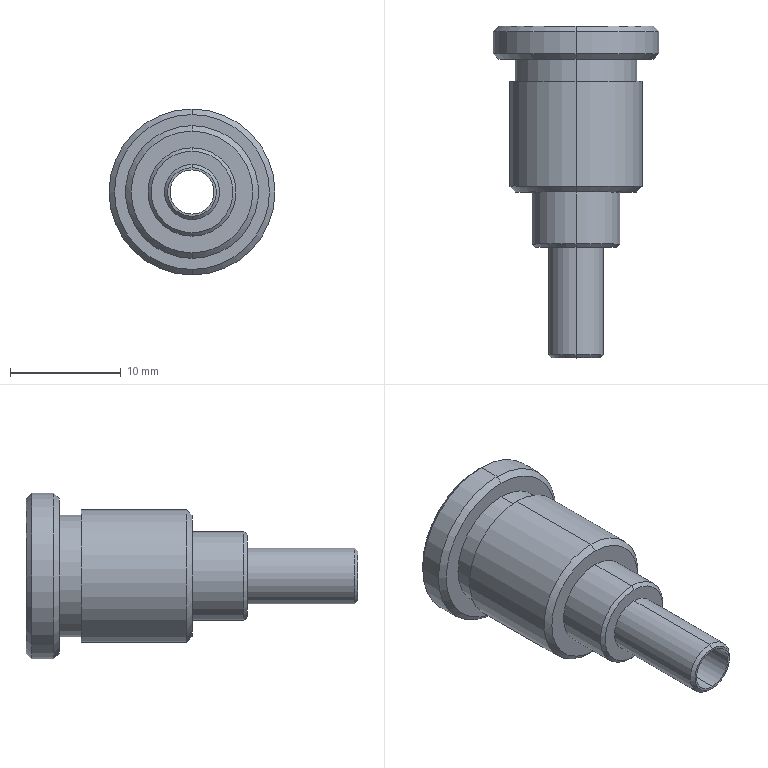Part | SolidWorks | features Chamfer 6, ICE 5, Extrusion 1, RevCut 1 | 1 solid | 30 faces | box 15 x 30 x 15 mm | volume 1897 mm3 | cylinder 12 | cone 12 | plane 6 | commonest cylinder face diameters 4 x2 5 x2 8 x2 11 x2 12 x2 15 x2
STEP:
#1=CARTESIAN_POINT('',(0.,-3.,-5.5));
#2=VERTEX_POINT('',#1);
#3=CARTESIAN_POINT('',(0.,-3.,5.5));
#4=VERTEX_POINT('',#3);
#5=CARTESIAN_POINT('',(0.,-3.,0.));
#6=DIRECTION('',(0.,-1.,0.));
#7=DIRECTION('',(0.,0.,-1.));
#8=AXIS2_PLACEMENT_3D('',#5,#6,#7);
#9=CIRCLE('',#8,5.5);
#10=EDGE_CURVE('',#2,#4,#9,.T.);
#11=ORIENTED_EDGE('',*,*,#10,.T.);
#12=CARTESIAN_POINT('',(0.,-5.,5.5));
#13=VERTEX_POINT('',#12);
#14=CARTESIAN_POINT('',(0.,-14.5,5.5));
#15=DIRECTION('',(0.,-1.,0.));
#16=VECTOR('',#15,1000.);
#17=LINE('',#14,#16);
#18=EDGE_CURVE('',#4,#13,#17,.T.);
#19=ORIENTED_EDGE('',*,*,#18,.T.);
#20=CARTESIAN_POINT('',(0.,-5.,-5.5));
#21=VERTEX_POINT('',#20);
#22=CARTESIAN_POINT('',(0.,-5.,0.));
#23=DIRECTION('',(0.,-1.,0.));
#24=DIRECTION('',(0.,0.,-1.));
#25=AXIS2_PLACEMENT_3D('',#22,#23,#24);
#26=CIRCLE('',#25,5.5);
#27=EDGE_CURVE('',#21,#13,#26,.T.);
#28=ORIENTED_EDGE('',*,*,#27,.F.);
#29=CARTESIAN_POINT('',(0.,-14.5,-5.5));
#30=DIRECTION('',(0.,-1.,0.));
#31=VECTOR('',#30,1000.);
#32=LINE('',#29,#31);
#33=EDGE_CURVE('',#2,#21,#32,.T.);
#34=ORIENTED_EDGE('',*,*,#33,.F.);
#35=EDGE_LOOP('',(#11,#19,#28,#34));
#36=FACE_OUTER_BOUND('',#35,.T.);
#37=CARTESIAN_POINT('',(0.,-14.5,0.));
#38=DIRECTION('',(0.,-1.,0.));
#39=DIRECTION('',(0.,0.,-1.));
#40=AXIS2_PLACEMENT_3D('',#37,#38,#39);
#41=CYLINDRICAL_SURFACE('',#40,5.5);
#42=ADVANCED_FACE('',(#36),#41,.T.);
#43=CARTESIAN_POINT('',(0.,-30.,-2.2));
#44=VERTEX_POINT('',#43);
#45=CARTESIAN_POINT('',(0.,-30.,2.2));
#46=VERTEX_POINT('',#45);
#47=CARTESIAN_POINT('',(0.,-30.,0.));
#48=DIRECTION('',(0.,-1.,0.));
#49=DIRECTION('',(0.,0.,-1.));
#50=AXIS2_PLACEMENT_3D('',#47,#48,#49);
#51=CIRCLE('',#50,2.2);
#52=EDGE_CURVE('',#44,#46,#51,.T.);
#53=ORIENTED_EDGE('',*,*,#52,.F.);
#54=CARTESIAN_POINT('',(0.,-29.7,-2.5));
#55=VERTEX_POINT('',#54);
#56=CARTESIAN_POINT('',(0.,-30.,-2.2));
#57=DIRECTION('',(0.,0.7071,-0.7071));
#58=VECTOR('',#57,1000.);
#59=LINE('',#56,#58);
#60=EDGE_CURVE('',#44,#55,#59,.T.);
#61=ORIENTED_EDGE('',*,*,#60,.T.);
#62=CARTESIAN_POINT('',(0.,-29.7,2.5));
#63=VERTEX_POINT('',#62);
#64=CARTESIAN_POINT('',(0.,-29.7,0.));
#65=DIRECTION('',(0.,1.,0.));
#66=DIRECTION('',(0.,0.,-1.));
#67=AXIS2_PLACEMENT_3D('',#64,#65,#66);
#68=CIRCLE('',#67,2.5);
#69=EDGE_CURVE('',#63,#55,#68,.T.);
#70=ORIENTED_EDGE('',*,*,#69,.F.);
#71=CARTESIAN_POINT('',(0.,-30.,2.2));
#72=DIRECTION('',(0.,0.7071,0.7071));
#73=VECTOR('',#72,1000.);
#74=LINE('',#71,#73);
#75=EDGE_CURVE('',#46,#63,#74,.T.);
#76=ORIENTED_EDGE('',*,*,#75,.F.);
#77=EDGE_LOOP('',(#53,#61,#70,#76));
#78=FACE_OUTER_BOUND('',#77,.T.);
#79=CARTESIAN_POINT('',(0.,-30.,0.));
#80=DIRECTION('',(0.,1.,0.));
#81=DIRECTION('',(0.,0.,1.));
#82=AXIS2_PLACEMENT_3D('',#79,#80,#81);
#83=CONICAL_SURFACE('',#82,2.2,0.7854);
#84=ADVANCED_FACE('',(#78),#83,.T.);
#85=CARTESIAN_POINT('',(0.,-20.,-3.7));
#86=VERTEX_POINT('',#85);
#87=CARTESIAN_POINT('',(0.,-20.,3.7));
#88=VERTEX_POINT('',#87);
#89=CARTESIAN_POINT('',(0.,-20.,0.));
#90=DIRECTION('',(0.,-1.,0.));
#91=DIRECTION('',(0.,0.,-1.));
#92=AXIS2_PLACEMENT_3D('',#89,#90,#91);
#93=CIRCLE('',#92,3.7);
#94=EDGE_CURVE('',#86,#88,#93,.T.);
#95=ORIENTED_EDGE('',*,*,#94,.F.);
#96=CARTESIAN_POINT('',(0.,-19.7,-4.));
#97=VERTEX_POINT('',#96);
#98=CARTESIAN_POINT('',(0.,-20.,-3.7));
#99=DIRECTION('',(0.,0.7071,-0.7071));
#100=VECTOR('',#99,1000.);
#101=LINE('',#98,#100);
#102=EDGE_CURVE('',#86,#97,#101,.T.);
#103=ORIENTED_EDGE('',*,*,#102,.T.);
#104=CARTESIAN_POINT('',(0.,-19.7,4.));
#105=VERTEX_POINT('',#104);
#106=CARTESIAN_POINT('',(0.,-19.7,0.));
#107=DIRECTION('',(0.,1.,0.));
#108=DIRECTION('',(0.,0.,-1.));
#109=AXIS2_PLACEMENT_3D('',#106,#107,#108);
#110=CIRCLE('',#109,4.);
#111=EDGE_CURVE('',#105,#97,#110,.T.);
#112=ORIENTED_EDGE('',*,*,#111,.F.);
#113=CARTESIAN_POINT('',(0.,-20.,3.7));
#114=DIRECTION('',(0.,0.7071,0.7071));
#115=VECTOR('',#114,1000.);
#116=LINE('',#113,#115);
#117=EDGE_CURVE('',#88,#105,#116,.T.);
#118=ORIENTED_EDGE('',*,*,#117,.F.);
#119=EDGE_LOOP('',(#95,#103,#112,#118));
#120=FACE_OUTER_BOUND('',#119,.T.);
#121=CARTESIAN_POINT('',(0.,-20.,0.));
#122=DIRECTION('',(0.,1.,0.));
#123=DIRECTION('',(0.,0.,1.));
#124=AXIS2_PLACEMENT_3D('',#121,#122,#123);
#125=CONICAL_SURFACE('',#124,3.7,0.7854);
#126=ADVANCED_FACE('',(#120),#125,.T.);
#127=ORIENTED_EDGE('',*,*,#111,.T.);
#128=CARTESIAN_POINT('',(0.,-15.,-4.));
#129=VERTEX_POINT('',#128);
#130=CARTESIAN_POINT('',(0.,-20.,-4.));
#131=DIRECTION('',(0.,1.,0.));
#132=VECTOR('',#131,1000.);
#133=LINE('',#130,#132);
#134=EDGE_CURVE('',#97,#129,#133,.T.);
#135=ORIENTED_EDGE('',*,*,#134,.T.);
#136=CARTESIAN_POINT('',(0.,-15.,4.));
#137=VERTEX_POINT('',#136);
#138=CARTESIAN_POINT('',(0.,-15.,0.));
#139=DIRECTION('',(0.,-1.,0.));
#140=DIRECTION('',(0.,0.,1.));
#141=AXIS2_PLACEMENT_3D('',#138,#139,#140);
#142=CIRCLE('',#141,4.);
#143=EDGE_CURVE('',#129,#137,#142,.T.);
#144=ORIENTED_EDGE('',*,*,#143,.T.);
#145=CARTESIAN_POINT('',(0.,-20.,4.));
#146=DIRECTION('',(0.,1.,0.));
#147=VECTOR('',#146,1000.);
#148=LINE('',#145,#147);
#149=EDGE_CURVE('',#105,#137,#148,.T.);
#150=ORIENTED_EDGE('',*,*,#149,.F.);
#151=EDGE_LOOP('',(#127,#135,#144,#150));
#152=FACE_OUTER_BOUND('',#151,.T.);
#153=CARTESIAN_POINT('',(0.,-20.,0.));
#154=DIRECTION('',(0.,1.,0.));
#155=DIRECTION('',(0.,0.,1.));
#156=AXIS2_PLACEMENT_3D('',#153,#154,#155);
#157=CYLINDRICAL_SURFACE('',#156,4.);
#158=ADVANCED_FACE('',(#152),#157,.T.);
#159=CARTESIAN_POINT('',(0.,-3.,-7.));
#160=VERTEX_POINT('',#159);
#161=CARTESIAN_POINT('',(0.,-3.,7.));
#162=VERTEX_POINT('',#161);
#163=CARTESIAN_POINT('',(0.,-3.,0.));
#164=DIRECTION('',(0.,-1.,0.));
#165=DIRECTION('',(0.,0.,1.));
#166=AXIS2_PLACEMENT_3D('',#163,#164,#165);
#167=CIRCLE('',#166,7.);
#168=EDGE_CURVE('',#160,#162,#167,.T.);
#169=ORIENTED_EDGE('',*,*,#168,.F.);
#170=CARTESIAN_POINT('',(0.,-2.5,-7.5));
#171=VERTEX_POINT('',#170);
#172=CARTESIAN_POINT('',(0.,-2.5,-7.5));
#173=DIRECTION('',(0.,0.7071,-0.7071));
#174=VECTOR('',#173,1000.);
#175=LINE('',#172,#174);
#176=EDGE_CURVE('',#160,#171,#175,.T.);
#177=ORIENTED_EDGE('',*,*,#176,.T.);
#178=CARTESIAN_POINT('',(0.,-2.5,7.5));
#179=VERTEX_POINT('',#178);
#180=CARTESIAN_POINT('',(0.,-2.5,0.));
#181=DIRECTION('',(0.,1.,0.));
#182=DIRECTION('',(0.,0.,1.));
#183=AXIS2_PLACEMENT_3D('',#180,#181,#182);
#184=CIRCLE('',#183,7.5);
#185=EDGE_CURVE('',#179,#171,#184,.T.);
#186=ORIENTED_EDGE('',*,*,#185,.F.);
#187=CARTESIAN_POINT('',(0.,-2.5,7.5));
#188=DIRECTION('',(0.,0.7071,0.7071));
#189=VECTOR('',#188,1000.);
#190=LINE('',#187,#189);
#191=EDGE_CURVE('',#162,#179,#190,.T.);
#192=ORIENTED_EDGE('',*,*,#191,.F.);
#193=EDGE_LOOP('',(#169,#177,#186,#192));
#194=FACE_OUTER_BOUND('',#193,.T.);
#195=CARTESIAN_POINT('',(0.,-2.5,0.));
#196=DIRECTION('',(0.,1.,0.));
#197=DIRECTION('',(0.,0.,1.));
#198=AXIS2_PLACEMENT_3D('',#195,#196,#197);
#199=CONICAL_SURFACE('',#198,7.5,0.7854);
#200=ADVANCED_FACE('',(#194),#199,.T.);
#201=CARTESIAN_POINT('',(0.,0.,7.));
#202=VERTEX_POINT('',#201);
#203=CARTESIAN_POINT('',(0.,0.,-7.));
#204=VERTEX_POINT('',#203);
#205=CARTESIAN_POINT('',(0.,0.,0.));
#206=DIRECTION('',(0.,1.,0.));
#207=DIRECTION('',(0.,0.,1.));
#208=AXIS2_PLACEMENT_3D('',#205,#206,#207);
#209=CIRCLE('',#208,7.);
#210=EDGE_CURVE('',#202,#204,#209,.T.);
#211=ORIENTED_EDGE('',*,*,#210,.F.);
#212=CARTESIAN_POINT('',(0.,-0.5,7.5));
#213=VERTEX_POINT('',#212);
#214=CARTESIAN_POINT('',(0.,0.,7.));
#215=DIRECTION('',(0.,-0.7071,0.7071));
#216=VECTOR('',#215,1000.);
#217=LINE('',#214,#216);
#218=EDGE_CURVE('',#202,#213,#217,.T.);
#219=ORIENTED_EDGE('',*,*,#218,.T.);
#220=CARTESIAN_POINT('',(0.,-0.5,-7.5));
#221=VERTEX_POINT('',#220);
#222=CARTESIAN_POINT('',(0.,-0.5,0.));
#223=DIRECTION('',(0.,-1.,0.));
#224=DIRECTION('',(0.,0.,1.));
#225=AXIS2_PLACEMENT_3D('',#222,#223,#224);
#226=CIRCLE('',#225,7.5);
#227=EDGE_CURVE('',#221,#213,#226,.T.);
#228=ORIENTED_EDGE('',*,*,#227,.F.);
#229=CARTESIAN_POINT('',(0.,0.,-7.));
#230=DIRECTION('',(0.,-0.7071,-0.7071));
#231=VECTOR('',#230,1000.);
#232=LINE('',#229,#231);
#233=EDGE_CURVE('',#204,#221,#232,.T.);
#234=ORIENTED_EDGE('',*,*,#233,.F.);
#235=EDGE_LOOP('',(#211,#219,#228,#234));
#236=FACE_OUTER_BOUND('',#235,.T.);
#237=CARTESIAN_POINT('',(0.,0.,0.));
#238=DIRECTION('',(0.,-1.,0.));
#239=DIRECTION('',(0.,0.,-1.));
#240=AXIS2_PLACEMENT_3D('',#237,#238,#239);
#241=CONICAL_SURFACE('',#240,7.,0.7854);
#242=ADVANCED_FACE('',(#236),#241,.T.);
#243=CARTESIAN_POINT('',(0.,-1.,-2.));
#244=VERTEX_POINT('',#243);
#245=CARTESIAN_POINT('',(0.,-1.,2.));
#246=VERTEX_POINT('',#245);
#247=CARTESIAN_POINT('',(0.,-1.,0.));
#248=DIRECTION('',(0.,1.,0.));
#249=DIRECTION('',(0.,0.,1.));
#250=AXIS2_PLACEMENT_3D('',#247,#248,#249);
#251=CIRCLE('',#250,2.);
#252=EDGE_CURVE('',#244,#246,#251,.T.);
#253=ORIENTED_EDGE('',*,*,#252,.F.);
#254=CARTESIAN_POINT('',(0.,0.,-3.));
#255=VERTEX_POINT('',#254);
#256=CARTESIAN_POINT('',(0.,-1.,-2.));
#257=DIRECTION('',(0.,0.7071,-0.7071));
#258=VECTOR('',#257,1000.);
#259=LINE('',#256,#258);
#260=EDGE_CURVE('',#244,#255,#259,.T.);
#261=ORIENTED_EDGE('',*,*,#260,.T.);
#262=CARTESIAN_POINT('',(0.,0.,3.));
#263=VERTEX_POINT('',#262);
#264=CARTESIAN_POINT('',(0.,0.,0.));
#265=DIRECTION('',(0.,-1.,0.));
#266=DIRECTION('',(0.,0.,1.));
#267=AXIS2_PLACEMENT_3D('',#264,#265,#266);
#268=CIRCLE('',#267,3.);
#269=EDGE_CURVE('',#263,#255,#268,.T.);
#270=ORIENTED_EDGE('',*,*,#269,.F.);
#271=CARTESIAN_POINT('',(0.,-1.,2.));
#272=DIRECTION('',(0.,0.7071,0.7071));
#273=VECTOR('',#272,1000.);
#274=LINE('',#271,#273);
#275=EDGE_CURVE('',#246,#263,#274,.T.);
#276=ORIENTED_EDGE('',*,*,#275,.F.);
#277=EDGE_LOOP('',(#253,#261,#270,#276));
#278=FACE_OUTER_BOUND('',#277,.T.);
#279=CARTESIAN_POINT('',(0.,-1.,0.));
#280=DIRECTION('',(0.,1.,0.));
#281=DIRECTION('',(0.,0.,1.));
#282=AXIS2_PLACEMENT_3D('',#279,#280,#281);
#283=CONICAL_SURFACE('',#282,2.,0.7854);
#284=ADVANCED_FACE('',(#278),#283,.F.);
#285=ORIENTED_EDGE('',*,*,#185,.T.);
#286=CARTESIAN_POINT('',(0.,-3.,-7.5));
#287=DIRECTION('',(0.,1.,0.));
#288=VECTOR('',#287,1000.);
#289=LINE('',#286,#288);
#290=EDGE_CURVE('',#171,#221,#289,.T.);
#291=ORIENTED_EDGE('',*,*,#290,.T.);
#292=ORIENTED_EDGE('',*,*,#227,.T.);
#293=CARTESIAN_POINT('',(0.,-3.,7.5));
#294=DIRECTION('',(0.,1.,0.));
#295=VECTOR('',#294,1000.);
#296=LINE('',#293,#295);
#297=EDGE_CURVE('',#179,#213,#296,.T.);
#298=ORIENTED_EDGE('',*,*,#297,.F.);
#299=EDGE_LOOP('',(#285,#291,#292,#298));
#300=FACE_OUTER_BOUND('',#299,.T.);
#301=CARTESIAN_POINT('',(0.,-3.,0.));
#302=DIRECTION('',(0.,1.,0.));
#303=DIRECTION('',(0.,0.,1.));
#304=AXIS2_PLACEMENT_3D('',#301,#302,#303);
#305=CYLINDRICAL_SURFACE('',#304,7.5);
#306=ADVANCED_FACE('',(#300),#305,.T.);
#307=CARTESIAN_POINT('',(0.,-15.,-5.5));
#308=VERTEX_POINT('',#307);
#309=CARTESIAN_POINT('',(0.,-15.,5.5));
#310=VERTEX_POINT('',#309);
#311=CARTESIAN_POINT('',(0.,-15.,0.));
#312=DIRECTION('',(0.,-1.,0.));
#313=DIRECTION('',(0.,0.,1.));
#314=AXIS2_PLACEMENT_3D('',#311,#312,#313);
#315=CIRCLE('',#314,5.5);
#316=EDGE_CURVE('',#308,#310,#315,.T.);
#317=ORIENTED_EDGE('',*,*,#316,.F.);
#318=CARTESIAN_POINT('',(0.,-14.5,-6.));
#319=VERTEX_POINT('',#318);
#320=CARTESIAN_POINT('',(0.,-14.5,-6.));
#321=DIRECTION('',(0.,0.7071,-0.7071));
#322=VECTOR('',#321,1000.);
#323=LINE('',#320,#322);
#324=EDGE_CURVE('',#308,#319,#323,.T.);
#325=ORIENTED_EDGE('',*,*,#324,.T.);
#326=CARTESIAN_POINT('',(0.,-14.5,6.));
#327=VERTEX_POINT('',#326);
#328=CARTESIAN_POINT('',(0.,-14.5,0.));
#329=DIRECTION('',(0.,1.,0.));
#330=DIRECTION('',(0.,0.,1.));
#331=AXIS2_PLACEMENT_3D('',#328,#329,#330);
#332=CIRCLE('',#331,6.);
#333=EDGE_CURVE('',#327,#319,#332,.T.);
#334=ORIENTED_EDGE('',*,*,#333,.F.);
#335=CARTESIAN_POINT('',(0.,-14.5,6.));
#336=DIRECTION('',(0.,0.7071,0.7071));
#337=VECTOR('',#336,1000.);
#338=LINE('',#335,#337);
#339=EDGE_CURVE('',#310,#327,#338,.T.);
#340=ORIENTED_EDGE('',*,*,#339,.F.);
#341=EDGE_LOOP('',(#317,#325,#334,#340));
#342=FACE_OUTER_BOUND('',#341,.T.);
#343=CARTESIAN_POINT('',(0.,-14.5,0.));
#344=DIRECTION('',(0.,1.,0.));
#345=DIRECTION('',(0.,0.,1.));
#346=AXIS2_PLACEMENT_3D('',#343,#344,#345);
#347=CONICAL_SURFACE('',#346,6.,0.7854);
#348=ADVANCED_FACE('',(#342),#347,.T.);
#349=CARTESIAN_POINT('',(0.,-30.,-2.));
#350=VERTEX_POINT('',#349);
#351=CARTESIAN_POINT('',(0.,-30.,2.));
#352=VERTEX_POINT('',#351);
#353=CARTESIAN_POINT('',(0.,-30.,0.));
#354=DIRECTION('',(0.,1.,0.));
#355=DIRECTION('',(0.,0.,1.));
#356=AXIS2_PLACEMENT_3D('',#353,#354,#355);
#357=CIRCLE('',#356,2.);
#358=EDGE_CURVE('',#350,#352,#357,.T.);
#359=ORIENTED_EDGE('',*,*,#358,.F.);
#360=CARTESIAN_POINT('',(0.,-30.,-2.));
#361=DIRECTION('',(0.,1.,0.));
#362=VECTOR('',#361,1000.);
#363=LINE('',#360,#362);
#364=EDGE_CURVE('',#350,#244,#363,.T.);
#365=ORIENTED_EDGE('',*,*,#364,.T.);
#366=ORIENTED_EDGE('',*,*,#252,.T.);
#367=CARTESIAN_POINT('',(0.,-30.,2.));
#368=DIRECTION('',(0.,1.,0.));
#369=VECTOR('',#368,1000.);
#370=LINE('',#367,#369);
#371=EDGE_CURVE('',#352,#246,#370,.T.);
#372=ORIENTED_EDGE('',*,*,#371,.F.);
#373=EDGE_LOOP('',(#359,#365,#366,#372));
#374=FACE_OUTER_BOUND('',#373,.T.);
#375=CARTESIAN_POINT('',(0.,-30.,0.));
#376=DIRECTION('',(0.,1.,0.));
#377=DIRECTION('',(0.,0.,1.));
#378=AXIS2_PLACEMENT_3D('',#375,#376,#377);
#379=CYLINDRICAL_SURFACE('',#378,2.);
#380=ADVANCED_FACE('',(#374),#379,.F.);
#381=ORIENTED_EDGE('',*,*,#69,.T.);
#382=CARTESIAN_POINT('',(0.,-20.,-2.5));
#383=VERTEX_POINT('',#382);
#384=CARTESIAN_POINT('',(0.,-30.,-2.5));
#385=DIRECTION('',(0.,1.,0.));
#386=VECTOR('',#385,1000.);
#387=LINE('',#384,#386);
#388=EDGE_CURVE('',#55,#383,#387,.T.);
#389=ORIENTED_EDGE('',*,*,#388,.T.);
#390=CARTESIAN_POINT('',(0.,-20.,2.5));
#391=VERTEX_POINT('',#390);
#392=CARTESIAN_POINT('',(0.,-20.,0.));
#393=DIRECTION('',(0.,-1.,0.));
#394=DIRECTION('',(0.,0.,-1.));
#395=AXIS2_PLACEMENT_3D('',#392,#393,#394);
#396=CIRCLE('',#395,2.5);
#397=EDGE_CURVE('',#383,#391,#396,.T.);
#398=ORIENTED_EDGE('',*,*,#397,.T.);
#399=CARTESIAN_POINT('',(0.,-30.,2.5));
#400=DIRECTION('',(0.,1.,0.));
#401=VECTOR('',#400,1000.);
#402=LINE('',#399,#401);
#403=EDGE_CURVE('',#63,#391,#402,.T.);
#404=ORIENTED_EDGE('',*,*,#403,.F.);
#405=EDGE_LOOP('',(#381,#389,#398,#404));
#406=FACE_OUTER_BOUND('',#405,.T.);
#407=CARTESIAN_POINT('',(0.,-30.,0.));
#408=DIRECTION('',(0.,1.,0.));
#409=DIRECTION('',(0.,0.,1.));
#410=AXIS2_PLACEMENT_3D('',#407,#408,#409);
#411=CYLINDRICAL_SURFACE('',#410,2.5);
#412=ADVANCED_FACE('',(#406),#411,.T.);
#413=ORIENTED_EDGE('',*,*,#333,.T.);
#414=CARTESIAN_POINT('',(0.,-5.,-6.));
#415=VERTEX_POINT('',#414);
#416=CARTESIAN_POINT('',(0.,-15.,-6.));
#417=DIRECTION('',(0.,1.,0.));
#418=VECTOR('',#417,1000.);
#419=LINE('',#416,#418);
#420=EDGE_CURVE('',#319,#415,#419,.T.);
#421=ORIENTED_EDGE('',*,*,#420,.T.);
#422=CARTESIAN_POINT('',(0.,-5.,6.));
#423=VERTEX_POINT('',#422);
#424=CARTESIAN_POINT('',(0.,-5.,0.));
#425=DIRECTION('',(0.,-1.,0.));
#426=DIRECTION('',(0.,0.,1.));
#427=AXIS2_PLACEMENT_3D('',#424,#425,#426);
#428=CIRCLE('',#427,6.);
#429=EDGE_CURVE('',#415,#423,#428,.T.);
#430=ORIENTED_EDGE('',*,*,#429,.T.);
#431=CARTESIAN_POINT('',(0.,-15.,6.));
#432=DIRECTION('',(0.,1.,0.));
#433=VECTOR('',#432,1000.);
#434=LINE('',#431,#433);
#435=EDGE_CURVE('',#327,#423,#434,.T.);
#436=ORIENTED_EDGE('',*,*,#435,.F.);
#437=EDGE_LOOP('',(#413,#421,#430,#436));
#438=FACE_OUTER_BOUND('',#437,.T.);
#439=CARTESIAN_POINT('',(0.,-15.,0.));
#440=DIRECTION('',(0.,1.,0.));
#441=DIRECTION('',(0.,0.,1.));
#442=AXIS2_PLACEMENT_3D('',#439,#440,#441);
#443=CYLINDRICAL_SURFACE('',#442,6.);
#444=ADVANCED_FACE('',(#438),#443,.T.);
#445=ORIENTED_EDGE('',*,*,#420,.F.);
#446=CARTESIAN_POINT('',(0.,-14.5,0.));
#447=DIRECTION('',(0.,1.,0.));
#448=DIRECTION('',(0.,0.,1.));
#449=AXIS2_PLACEMENT_3D('',#446,#447,#448);
#450=CIRCLE('',#449,6.);
#451=EDGE_CURVE('',#319,#327,#450,.T.);
#452=ORIENTED_EDGE('',*,*,#451,.T.);
#453=ORIENTED_EDGE('',*,*,#435,.T.);
#454=CARTESIAN_POINT('',(0.,-5.,0.));
#455=DIRECTION('',(0.,-1.,0.));
#456=DIRECTION('',(0.,0.,1.));
#457=AXIS2_PLACEMENT_3D('',#454,#455,#456);
#458=CIRCLE('',#457,6.);
#459=EDGE_CURVE('',#423,#415,#458,.T.);
#460=ORIENTED_EDGE('',*,*,#459,.T.);
#461=EDGE_LOOP('',(#445,#452,#453,#460));
#462=FACE_OUTER_BOUND('',#461,.T.);
#463=CARTESIAN_POINT('',(0.,-15.,0.));
#464=DIRECTION('',(0.,1.,0.));
#465=DIRECTION('',(0.,0.,1.));
#466=AXIS2_PLACEMENT_3D('',#463,#464,#465);
#467=CYLINDRICAL_SURFACE('',#466,6.);
#468=ADVANCED_FACE('',(#462),#467,.T.);
#469=CARTESIAN_POINT('',(0.,-15.,0.));
#470=DIRECTION('',(0.,-1.,0.));
#471=DIRECTION('',(0.,0.,1.));
#472=AXIS2_PLACEMENT_3D('',#469,#470,#471);
#473=CIRCLE('',#472,5.5);
#474=EDGE_CURVE('',#310,#308,#473,.T.);
#475=ORIENTED_EDGE('',*,*,#474,.T.);
#476=ORIENTED_EDGE('',*,*,#316,.T.);
#477=EDGE_LOOP('',(#475,#476));
#478=FACE_OUTER_BOUND('',#477,.T.);
#479=CARTESIAN_POINT('',(0.,-15.,0.));
#480=DIRECTION('',(0.,-1.,0.));
#481=DIRECTION('',(0.,0.,1.));
#482=AXIS2_PLACEMENT_3D('',#479,#480,#481);
#483=CIRCLE('',#482,4.);
#484=EDGE_CURVE('',#137,#129,#483,.T.);
#485=ORIENTED_EDGE('',*,*,#484,.F.);
#486=ORIENTED_EDGE('',*,*,#143,.F.);
#487=EDGE_LOOP('',(#485,#486));
#488=FACE_BOUND('',#487,.T.);
#489=CARTESIAN_POINT('',(0.,-15.,0.));
#490=DIRECTION('',(0.,1.,0.));
#491=DIRECTION('',(0.,0.,1.));
#492=AXIS2_PLACEMENT_3D('',#489,#490,#491);
#493=PLANE('',#492);
#494=ADVANCED_FACE('',(#478,#488),#493,.F.);
#495=CARTESIAN_POINT('',(0.,0.,0.));
#496=DIRECTION('',(0.,1.,0.));
#497=DIRECTION('',(0.,0.,1.));
#498=AXIS2_PLACEMENT_3D('',#495,#496,#497);
#499=CIRCLE('',#498,7.);
#500=EDGE_CURVE('',#204,#202,#499,.T.);
#501=ORIENTED_EDGE('',*,*,#500,.T.);
#502=ORIENTED_EDGE('',*,*,#210,.T.);
#503=EDGE_LOOP('',(#501,#502));
#504=FACE_OUTER_BOUND('',#503,.T.);
#505=ORIENTED_EDGE('',*,*,#269,.T.);
#506=CARTESIAN_POINT('',(0.,0.,0.));
#507=DIRECTION('',(0.,-1.,0.));
#508=DIRECTION('',(0.,0.,1.));
#509=AXIS2_PLACEMENT_3D('',#506,#507,#508);
#510=CIRCLE('',#509,3.);
#511=EDGE_CURVE('',#255,#263,#510,.T.);
#512=ORIENTED_EDGE('',*,*,#511,.T.);
#513=EDGE_LOOP('',(#505,#512));
#514=FACE_BOUND('',#513,.T.);
#515=CARTESIAN_POINT('',(0.,0.,0.));
#516=DIRECTION('',(0.,1.,0.));
#517=DIRECTION('',(0.,0.,1.));
#518=AXIS2_PLACEMENT_3D('',#515,#516,#517);
#519=PLANE('',#518);
#520=ADVANCED_FACE('',(#504,#514),#519,.T.);
#521=ORIENTED_EDGE('',*,*,#388,.F.);
#522=CARTESIAN_POINT('',(0.,-29.7,0.));
#523=DIRECTION('',(0.,1.,0.));
#524=DIRECTION('',(0.,0.,-1.));
#525=AXIS2_PLACEMENT_3D('',#522,#523,#524);
#526=CIRCLE('',#525,2.5);
#527=EDGE_CURVE('',#55,#63,#526,.T.);
#528=ORIENTED_EDGE('',*,*,#527,.T.);
#529=ORIENTED_EDGE('',*,*,#403,.T.);
#530=CARTESIAN_POINT('',(0.,-20.,0.));
#531=DIRECTION('',(0.,-1.,0.));
#532=DIRECTION('',(0.,0.,-1.));
#533=AXIS2_PLACEMENT_3D('',#530,#531,#532);
#534=CIRCLE('',#533,2.5);
#535=EDGE_CURVE('',#391,#383,#534,.T.);
#536=ORIENTED_EDGE('',*,*,#535,.T.);
#537=EDGE_LOOP('',(#521,#528,#529,#536));
#538=FACE_OUTER_BOUND('',#537,.T.);
#539=CARTESIAN_POINT('',(0.,-30.,0.));
#540=DIRECTION('',(0.,1.,0.));
#541=DIRECTION('',(0.,0.,1.));
#542=AXIS2_PLACEMENT_3D('',#539,#540,#541);
#543=CYLINDRICAL_SURFACE('',#542,2.5);
#544=ADVANCED_FACE('',(#538),#543,.T.);
#545=CARTESIAN_POINT('',(0.,-30.,0.));
#546=DIRECTION('',(0.,-1.,0.));
#547=DIRECTION('',(0.,0.,-1.));
#548=AXIS2_PLACEMENT_3D('',#545,#546,#547);
#549=CIRCLE('',#548,2.2);
#550=EDGE_CURVE('',#46,#44,#549,.T.);
#551=ORIENTED_EDGE('',*,*,#550,.T.);
#552=ORIENTED_EDGE('',*,*,#52,.T.);
#553=EDGE_LOOP('',(#551,#552));
#554=FACE_OUTER_BOUND('',#553,.T.);
#555=CARTESIAN_POINT('',(0.,-30.,0.));
#556=DIRECTION('',(0.,1.,0.));
#557=DIRECTION('',(0.,0.,1.));
#558=AXIS2_PLACEMENT_3D('',#555,#556,#557);
#559=CIRCLE('',#558,2.);
#560=EDGE_CURVE('',#352,#350,#559,.T.);
#561=ORIENTED_EDGE('',*,*,#560,.T.);
#562=ORIENTED_EDGE('',*,*,#358,.T.);
#563=EDGE_LOOP('',(#561,#562));
#564=FACE_BOUND('',#563,.T.);
#565=CARTESIAN_POINT('',(0.,-30.,0.));
#566=DIRECTION('',(0.,-1.,0.));
#567=DIRECTION('',(0.,0.,-1.));
#568=AXIS2_PLACEMENT_3D('',#565,#566,#567);
#569=PLANE('',#568);
#570=ADVANCED_FACE('',(#554,#564),#569,.T.);
#571=ORIENTED_EDGE('',*,*,#364,.F.);
#572=ORIENTED_EDGE('',*,*,#560,.F.);
#573=ORIENTED_EDGE('',*,*,#371,.T.);
#574=CARTESIAN_POINT('',(0.,-1.,0.));
#575=DIRECTION('',(0.,1.,0.));
#576=DIRECTION('',(0.,0.,1.));
#577=AXIS2_PLACEMENT_3D('',#574,#575,#576);
#578=CIRCLE('',#577,2.);
#579=EDGE_CURVE('',#246,#244,#578,.T.);
#580=ORIENTED_EDGE('',*,*,#579,.T.);
#581=EDGE_LOOP('',(#571,#572,#573,#580));
#582=FACE_OUTER_BOUND('',#581,.T.);
#583=CARTESIAN_POINT('',(0.,-30.,0.));
#584=DIRECTION('',(0.,1.,0.));
#585=DIRECTION('',(0.,0.,1.));
#586=AXIS2_PLACEMENT_3D('',#583,#584,#585);
#587=CYLINDRICAL_SURFACE('',#586,2.);
#588=ADVANCED_FACE('',(#582),#587,.F.);
#589=ORIENTED_EDGE('',*,*,#324,.F.);
#590=ORIENTED_EDGE('',*,*,#474,.F.);
#591=ORIENTED_EDGE('',*,*,#339,.T.);
#592=ORIENTED_EDGE('',*,*,#451,.F.);
#593=EDGE_LOOP('',(#589,#590,#591,#592));
#594=FACE_OUTER_BOUND('',#593,.T.);
#595=CARTESIAN_POINT('',(0.,-14.5,0.));
#596=DIRECTION('',(0.,1.,0.));
#597=DIRECTION('',(0.,0.,1.));
#598=AXIS2_PLACEMENT_3D('',#595,#596,#597);
#599=CONICAL_SURFACE('',#598,6.,0.7854);
#600=ADVANCED_FACE('',(#594),#599,.T.);
#601=ORIENTED_EDGE('',*,*,#290,.F.);
#602=CARTESIAN_POINT('',(0.,-2.5,0.));
#603=DIRECTION('',(0.,1.,0.));
#604=DIRECTION('',(0.,0.,1.));
#605=AXIS2_PLACEMENT_3D('',#602,#603,#604);
#606=CIRCLE('',#605,7.5);
#607=EDGE_CURVE('',#171,#179,#606,.T.);
#608=ORIENTED_EDGE('',*,*,#607,.T.);
#609=ORIENTED_EDGE('',*,*,#297,.T.);
#610=CARTESIAN_POINT('',(0.,-0.5,0.));
#611=DIRECTION('',(0.,-1.,0.));
#612=DIRECTION('',(0.,0.,1.));
#613=AXIS2_PLACEMENT_3D('',#610,#611,#612);
#614=CIRCLE('',#613,7.5);
#615=EDGE_CURVE('',#213,#221,#614,.T.);
#616=ORIENTED_EDGE('',*,*,#615,.T.);
#617=EDGE_LOOP('',(#601,#608,#609,#616));
#618=FACE_OUTER_BOUND('',#617,.T.);
#619=CARTESIAN_POINT('',(0.,-3.,0.));
#620=DIRECTION('',(0.,1.,0.));
#621=DIRECTION('',(0.,0.,1.));
#622=AXIS2_PLACEMENT_3D('',#619,#620,#621);
#623=CYLINDRICAL_SURFACE('',#622,7.5);
#624=ADVANCED_FACE('',(#618),#623,.T.);
#625=CARTESIAN_POINT('',(0.,-3.,0.));
#626=DIRECTION('',(0.,-1.,0.));
#627=DIRECTION('',(0.,0.,1.));
#628=AXIS2_PLACEMENT_3D('',#625,#626,#627);
#629=CIRCLE('',#628,7.);
#630=EDGE_CURVE('',#162,#160,#629,.T.);
#631=ORIENTED_EDGE('',*,*,#630,.T.);
#632=ORIENTED_EDGE('',*,*,#168,.T.);
#633=EDGE_LOOP('',(#631,#632));
#634=FACE_OUTER_BOUND('',#633,.T.);
#635=ORIENTED_EDGE('',*,*,#10,.F.);
#636=CARTESIAN_POINT('',(0.,-3.,0.));
#637=DIRECTION('',(0.,-1.,0.));
#638=DIRECTION('',(0.,0.,-1.));
#639=AXIS2_PLACEMENT_3D('',#636,#637,#638);
#640=CIRCLE('',#639,5.5);
#641=EDGE_CURVE('',#4,#2,#640,.T.);
#642=ORIENTED_EDGE('',*,*,#641,.F.);
#643=EDGE_LOOP('',(#635,#642));
#644=FACE_BOUND('',#643,.T.);
#645=CARTESIAN_POINT('',(0.,-3.,0.));
#646=DIRECTION('',(0.,1.,0.));
#647=DIRECTION('',(0.,0.,1.));
#648=AXIS2_PLACEMENT_3D('',#645,#646,#647);
#649=PLANE('',#648);
#650=ADVANCED_FACE('',(#634,#644),#649,.F.);
#651=ORIENTED_EDGE('',*,*,#260,.F.);
#652=ORIENTED_EDGE('',*,*,#579,.F.);
#653=ORIENTED_EDGE('',*,*,#275,.T.);
#654=ORIENTED_EDGE('',*,*,#511,.F.);
#655=EDGE_LOOP('',(#651,#652,#653,#654));
#656=FACE_OUTER_BOUND('',#655,.T.);
#657=CARTESIAN_POINT('',(0.,-1.,0.));
#658=DIRECTION('',(0.,1.,0.));
#659=DIRECTION('',(0.,0.,1.));
#660=AXIS2_PLACEMENT_3D('',#657,#658,#659);
#661=CONICAL_SURFACE('',#660,2.,0.7854);
#662=ADVANCED_FACE('',(#656),#661,.F.);
#663=ORIENTED_EDGE('',*,*,#218,.F.);
#664=ORIENTED_EDGE('',*,*,#500,.F.);
#665=ORIENTED_EDGE('',*,*,#233,.T.);
#666=ORIENTED_EDGE('',*,*,#615,.F.);
#667=EDGE_LOOP('',(#663,#664,#665,#666));
#668=FACE_OUTER_BOUND('',#667,.T.);
#669=CARTESIAN_POINT('',(0.,0.,0.));
#670=DIRECTION('',(0.,-1.,0.));
#671=DIRECTION('',(0.,0.,-1.));
#672=AXIS2_PLACEMENT_3D('',#669,#670,#671);
#673=CONICAL_SURFACE('',#672,7.,0.7854);
#674=ADVANCED_FACE('',(#668),#673,.T.);
#675=ORIENTED_EDGE('',*,*,#176,.F.);
#676=ORIENTED_EDGE('',*,*,#630,.F.);
#677=ORIENTED_EDGE('',*,*,#191,.T.);
#678=ORIENTED_EDGE('',*,*,#607,.F.);
#679=EDGE_LOOP('',(#675,#676,#677,#678));
#680=FACE_OUTER_BOUND('',#679,.T.);
#681=CARTESIAN_POINT('',(0.,-2.5,0.));
#682=DIRECTION('',(0.,1.,0.));
#683=DIRECTION('',(0.,0.,1.));
#684=AXIS2_PLACEMENT_3D('',#681,#682,#683);
#685=CONICAL_SURFACE('',#684,7.5,0.7854);
#686=ADVANCED_FACE('',(#680),#685,.T.);
#687=CARTESIAN_POINT('',(0.,-20.,0.));
#688=DIRECTION('',(0.,-1.,0.));
#689=DIRECTION('',(0.,0.,-1.));
#690=AXIS2_PLACEMENT_3D('',#687,#688,#689);
#691=CIRCLE('',#690,3.7);
#692=EDGE_CURVE('',#88,#86,#691,.T.);
#693=ORIENTED_EDGE('',*,*,#692,.T.);
#694=ORIENTED_EDGE('',*,*,#94,.T.);
#695=EDGE_LOOP('',(#693,#694));
#696=FACE_OUTER_BOUND('',#695,.T.);
#697=ORIENTED_EDGE('',*,*,#535,.F.);
#698=ORIENTED_EDGE('',*,*,#397,.F.);
#699=EDGE_LOOP('',(#697,#698));
#700=FACE_BOUND('',#699,.T.);
#701=CARTESIAN_POINT('',(0.,-20.,0.));
#702=DIRECTION('',(0.,-1.,0.));
#703=DIRECTION('',(0.,0.,-1.));
#704=AXIS2_PLACEMENT_3D('',#701,#702,#703);
#705=PLANE('',#704);
#706=ADVANCED_FACE('',(#696,#700),#705,.T.);
#707=ORIENTED_EDGE('',*,*,#134,.F.);
#708=CARTESIAN_POINT('',(0.,-19.7,0.));
#709=DIRECTION('',(0.,1.,0.));
#710=DIRECTION('',(0.,0.,-1.));
#711=AXIS2_PLACEMENT_3D('',#708,#709,#710);
#712=CIRCLE('',#711,4.);
#713=EDGE_CURVE('',#97,#105,#712,.T.);
#714=ORIENTED_EDGE('',*,*,#713,.T.);
#715=ORIENTED_EDGE('',*,*,#149,.T.);
#716=ORIENTED_EDGE('',*,*,#484,.T.);
#717=EDGE_LOOP('',(#707,#714,#715,#716));
#718=FACE_OUTER_BOUND('',#717,.T.);
#719=CARTESIAN_POINT('',(0.,-20.,0.));
#720=DIRECTION('',(0.,1.,0.));
#721=DIRECTION('',(0.,0.,1.));
#722=AXIS2_PLACEMENT_3D('',#719,#720,#721);
#723=CYLINDRICAL_SURFACE('',#722,4.);
#724=ADVANCED_FACE('',(#718),#723,.T.);
#725=ORIENTED_EDGE('',*,*,#102,.F.);
#726=ORIENTED_EDGE('',*,*,#692,.F.);
#727=ORIENTED_EDGE('',*,*,#117,.T.);
#728=ORIENTED_EDGE('',*,*,#713,.F.);
#729=EDGE_LOOP('',(#725,#726,#727,#728));
#730=FACE_OUTER_BOUND('',#729,.T.);
#731=CARTESIAN_POINT('',(0.,-20.,0.));
#732=DIRECTION('',(0.,1.,0.));
#733=DIRECTION('',(0.,0.,1.));
#734=AXIS2_PLACEMENT_3D('',#731,#732,#733);
#735=CONICAL_SURFACE('',#734,3.7,0.7854);
#736=ADVANCED_FACE('',(#730),#735,.T.);
#737=ORIENTED_EDGE('',*,*,#60,.F.);
#738=ORIENTED_EDGE('',*,*,#550,.F.);
#739=ORIENTED_EDGE('',*,*,#75,.T.);
#740=ORIENTED_EDGE('',*,*,#527,.F.);
#741=EDGE_LOOP('',(#737,#738,#739,#740));
#742=FACE_OUTER_BOUND('',#741,.T.);
#743=CARTESIAN_POINT('',(0.,-30.,0.));
#744=DIRECTION('',(0.,1.,0.));
#745=DIRECTION('',(0.,0.,1.));
#746=AXIS2_PLACEMENT_3D('',#743,#744,#745);
#747=CONICAL_SURFACE('',#746,2.2,0.7854);
#748=ADVANCED_FACE('',(#742),#747,.T.);
#749=ORIENTED_EDGE('',*,*,#18,.F.);
#750=ORIENTED_EDGE('',*,*,#641,.T.);
#751=ORIENTED_EDGE('',*,*,#33,.T.);
#752=CARTESIAN_POINT('',(0.,-5.,0.));
#753=DIRECTION('',(0.,-1.,0.));
#754=DIRECTION('',(0.,0.,-1.));
#755=AXIS2_PLACEMENT_3D('',#752,#753,#754);
#756=CIRCLE('',#755,5.5);
#757=EDGE_CURVE('',#13,#21,#756,.T.);
#758=ORIENTED_EDGE('',*,*,#757,.F.);
#759=EDGE_LOOP('',(#749,#750,#751,#758));
#760=FACE_OUTER_BOUND('',#759,.T.);
#761=CARTESIAN_POINT('',(0.,-14.5,0.));
#762=DIRECTION('',(0.,-1.,0.));
#763=DIRECTION('',(0.,0.,-1.));
#764=AXIS2_PLACEMENT_3D('',#761,#762,#763);
#765=CYLINDRICAL_SURFACE('',#764,5.5);
#766=ADVANCED_FACE('',(#760),#765,.T.);
#767=ORIENTED_EDGE('',*,*,#459,.F.);
#768=ORIENTED_EDGE('',*,*,#429,.F.);
#769=EDGE_LOOP('',(#767,#768));
#770=FACE_OUTER_BOUND('',#769,.T.);
#771=ORIENTED_EDGE('',*,*,#27,.T.);
#772=ORIENTED_EDGE('',*,*,#757,.T.);
#773=EDGE_LOOP('',(#771,#772));
#774=FACE_BOUND('',#773,.T.);
#775=CARTESIAN_POINT('',(-8.868,-5.,0.));
#776=DIRECTION('',(0.,1.,0.));
#777=DIRECTION('',(0.,0.,1.));
#778=AXIS2_PLACEMENT_3D('',#775,#776,#777);
#779=PLANE('',#778);
#780=ADVANCED_FACE('',(#770,#774),#779,.T.);
#781=CLOSED_SHELL('',(#42,#84,#126,#158,#200,#242,#284,#306,#348,#380,#412,#444,#468,#494,#520,#544,#570,#588,#600,#624,#650,#662,#674,#686,#706,#724,#736,#748,#766,#780));
#782=MANIFOLD_SOLID_BREP('',#781);
#783=CARTESIAN_POINT('',(0.,0.,0.));
#784=DIRECTION('',(0.,0.,1.));
#785=DIRECTION('',(1.,0.,0.));
#786=AXIS2_PLACEMENT_3D('',#783,#784,#785);
#787=(LENGTH_UNIT()NAMED_UNIT(*)SI_UNIT(.MILLI.,.METRE.));
#788=UNCERTAINTY_MEASURE_WITH_UNIT(LENGTH_MEASURE(0.00001),#787,'','');
#789=(NAMED_UNIT(*)PLANE_ANGLE_UNIT()SI_UNIT($,.RADIAN.));
#790=(NAMED_UNIT(*)SI_UNIT($,.STERADIAN.)SOLID_ANGLE_UNIT());
#791=(GEOMETRIC_REPRESENTATION_CONTEXT(3)GLOBAL_UNCERTAINTY_ASSIGNED_CONTEXT((#788))GLOBAL_UNIT_ASSIGNED_CONTEXT((#787,#789,#790))REPRESENTATION_CONTEXT('',''));
#792=ADVANCED_BREP_SHAPE_REPRESENTATION('',(#782,#786),#791);